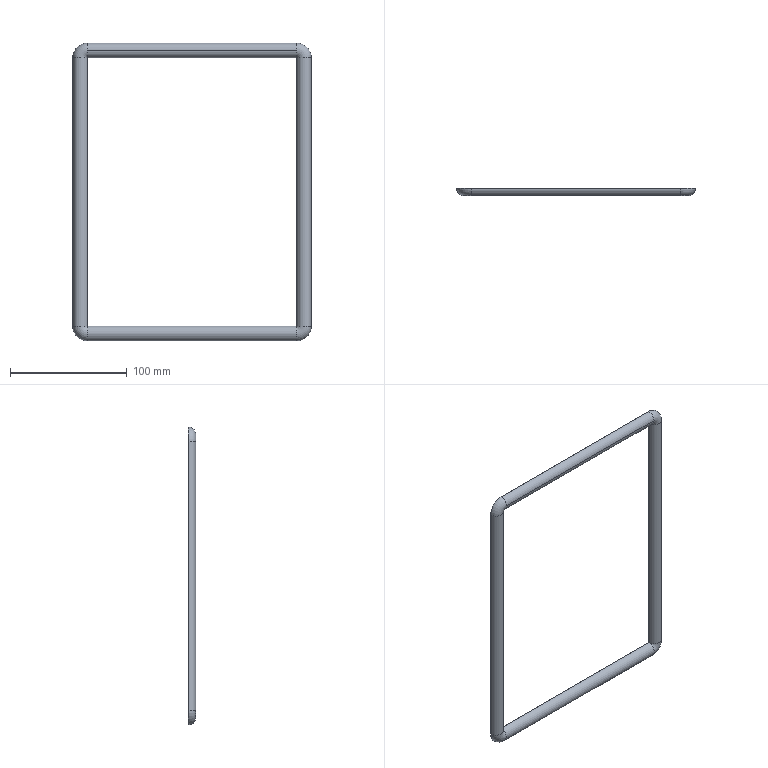Part | SolidWorks | features BaseBody 1 | 1 solid | 43 faces | box 204.775 x 6.35 x 255.575 mm | volume 53856 mm3 | plane 18 | cylinder 13 | cone 8 | torus 4 | commonest cylinder face diameters 12.7 x5 0.051 x4 25.349 x4
STEP:
#1=CARTESIAN_POINT('',(-89.687,-6.35,121.437));
#2=VERTEX_POINT('',#1);
#3=CARTESIAN_POINT('',(-89.687,0.,127.787));
#4=VERTEX_POINT('',#3);
#5=CARTESIAN_POINT('',(-89.687,0.,121.437));
#6=DIRECTION('',(-1.,0.,0.));
#7=DIRECTION('',(0.,0.,-1.));
#8=AXIS2_PLACEMENT_3D('',#5,#6,#7);
#9=CIRCLE('',#8,6.35);
#10=EDGE_CURVE('',#2,#4,#9,.T.);
#11=ORIENTED_EDGE('',*,*,#10,.F.);
#12=CARTESIAN_POINT('',(89.687,-6.35,121.437));
#13=VERTEX_POINT('',#12);
#14=CARTESIAN_POINT('',(-89.687,-6.35,121.437));
#15=DIRECTION('',(1.,0.,0.));
#16=VECTOR('',#15,1000.);
#17=LINE('',#14,#16);
#18=EDGE_CURVE('',#2,#13,#17,.T.);
#19=ORIENTED_EDGE('',*,*,#18,.T.);
#20=CARTESIAN_POINT('',(89.687,0.,127.787));
#21=VERTEX_POINT('',#20);
#22=CARTESIAN_POINT('',(89.687,0.,121.437));
#23=DIRECTION('',(-1.,0.,0.));
#24=DIRECTION('',(0.,0.,-1.));
#25=AXIS2_PLACEMENT_3D('',#22,#23,#24);
#26=CIRCLE('',#25,6.35);
#27=EDGE_CURVE('',#13,#21,#26,.T.);
#28=ORIENTED_EDGE('',*,*,#27,.T.);
#29=CARTESIAN_POINT('',(-89.687,0.,127.787));
#30=DIRECTION('',(1.,0.,0.));
#31=VECTOR('',#30,1000.);
#32=LINE('',#29,#31);
#33=EDGE_CURVE('',#4,#21,#32,.T.);
#34=ORIENTED_EDGE('',*,*,#33,.F.);
#35=EDGE_LOOP('',(#11,#19,#28,#34));
#36=FACE_OUTER_BOUND('',#35,.T.);
#37=CARTESIAN_POINT('',(-89.687,0.,121.437));
#38=DIRECTION('',(1.,0.,0.));
#39=DIRECTION('',(0.,-1.,0.));
#40=AXIS2_PLACEMENT_3D('',#37,#38,#39);
#41=CYLINDRICAL_SURFACE('',#40,6.35);
#42=ADVANCED_FACE('',(#36),#41,.T.);
#43=CARTESIAN_POINT('',(-89.687,0.,-115.087));
#44=VERTEX_POINT('',#43);
#45=CARTESIAN_POINT('',(-89.687,0.,-127.787));
#46=VERTEX_POINT('',#45);
#47=CARTESIAN_POINT('',(-89.687,0.,-121.437));
#48=DIRECTION('',(1.,0.,0.));
#49=DIRECTION('',(0.,0.,1.));
#50=AXIS2_PLACEMENT_3D('',#47,#48,#49);
#51=CIRCLE('',#50,6.35);
#52=EDGE_CURVE('',#44,#46,#51,.T.);
#53=ORIENTED_EDGE('',*,*,#52,.F.);
#54=CARTESIAN_POINT('',(-102.387,0.,-115.087));
#55=VERTEX_POINT('',#54);
#56=CARTESIAN_POINT('',(-96.037,0.,-115.087));
#57=DIRECTION('',(0.,0.,-1.));
#58=DIRECTION('',(1.,0.,0.));
#59=AXIS2_PLACEMENT_3D('',#56,#57,#58);
#60=CIRCLE('',#59,6.35);
#61=EDGE_CURVE('',#44,#55,#60,.T.);
#62=ORIENTED_EDGE('',*,*,#61,.T.);
#63=CARTESIAN_POINT('',(-89.687,0.,-115.087));
#64=DIRECTION('',(0.,1.,0.));
#65=DIRECTION('',(0.,0.,-1.));
#66=AXIS2_PLACEMENT_3D('',#63,#64,#65);
#67=CIRCLE('',#66,12.7);
#68=EDGE_CURVE('',#46,#55,#67,.T.);
#69=ORIENTED_EDGE('',*,*,#68,.F.);
#70=EDGE_LOOP('',(#53,#62,#69));
#71=FACE_OUTER_BOUND('',#70,.T.);
#72=CARTESIAN_POINT('',(-89.687,0.,-115.087));
#73=DIRECTION('',(0.,1.,0.));
#74=DIRECTION('',(1.,0.,0.));
#75=AXIS2_PLACEMENT_3D('',#72,#73,#74);
#76=TOROIDAL_SURFACE('',#75,6.35,6.35);
#77=ADVANCED_FACE('',(#71),#76,.T.);
#78=CARTESIAN_POINT('',(89.687,0.,-115.087));
#79=VERTEX_POINT('',#78);
#80=CARTESIAN_POINT('',(89.687,0.,-115.087));
#81=DIRECTION('',(-1.,0.,0.));
#82=VECTOR('',#81,1000.);
#83=LINE('',#80,#82);
#84=EDGE_CURVE('',#79,#44,#83,.T.);
#85=ORIENTED_EDGE('',*,*,#84,.T.);
#86=ORIENTED_EDGE('',*,*,#52,.T.);
#87=CARTESIAN_POINT('',(89.687,0.,-127.787));
#88=VERTEX_POINT('',#87);
#89=CARTESIAN_POINT('',(89.687,0.,-127.787));
#90=DIRECTION('',(-1.,0.,0.));
#91=VECTOR('',#90,1000.);
#92=LINE('',#89,#91);
#93=EDGE_CURVE('',#88,#46,#92,.T.);
#94=ORIENTED_EDGE('',*,*,#93,.F.);
#95=CARTESIAN_POINT('',(89.687,0.,-121.437));
#96=DIRECTION('',(1.,0.,0.));
#97=DIRECTION('',(0.,0.,1.));
#98=AXIS2_PLACEMENT_3D('',#95,#96,#97);
#99=CIRCLE('',#98,6.35);
#100=EDGE_CURVE('',#79,#88,#99,.T.);
#101=ORIENTED_EDGE('',*,*,#100,.F.);
#102=EDGE_LOOP('',(#85,#86,#94,#101));
#103=FACE_OUTER_BOUND('',#102,.T.);
#104=CARTESIAN_POINT('',(89.687,0.,-121.437));
#105=DIRECTION('',(-1.,0.,0.));
#106=DIRECTION('',(0.,0.,1.));
#107=AXIS2_PLACEMENT_3D('',#104,#105,#106);
#108=CYLINDRICAL_SURFACE('',#107,6.35);
#109=ADVANCED_FACE('',(#103),#108,.T.);
#110=CARTESIAN_POINT('',(102.387,0.,-115.087));
#111=VERTEX_POINT('',#110);
#112=CARTESIAN_POINT('',(96.037,0.,-115.087));
#113=DIRECTION('',(0.,0.,1.));
#114=DIRECTION('',(-1.,0.,0.));
#115=AXIS2_PLACEMENT_3D('',#112,#113,#114);
#116=CIRCLE('',#115,6.35);
#117=EDGE_CURVE('',#79,#111,#116,.T.);
#118=ORIENTED_EDGE('',*,*,#117,.F.);
#119=ORIENTED_EDGE('',*,*,#100,.T.);
#120=CARTESIAN_POINT('',(89.687,0.,-115.087));
#121=DIRECTION('',(0.,1.,0.));
#122=DIRECTION('',(1.,0.,0.));
#123=AXIS2_PLACEMENT_3D('',#120,#121,#122);
#124=CIRCLE('',#123,12.7);
#125=EDGE_CURVE('',#111,#88,#124,.T.);
#126=ORIENTED_EDGE('',*,*,#125,.F.);
#127=EDGE_LOOP('',(#118,#119,#126));
#128=FACE_OUTER_BOUND('',#127,.T.);
#129=CARTESIAN_POINT('',(89.687,0.,-115.087));
#130=DIRECTION('',(0.,1.,0.));
#131=DIRECTION('',(1.,0.,0.));
#132=AXIS2_PLACEMENT_3D('',#129,#130,#131);
#133=TOROIDAL_SURFACE('',#132,6.35,6.35);
#134=ADVANCED_FACE('',(#128),#133,.T.);
#135=CARTESIAN_POINT('',(89.687,0.,115.087));
#136=VERTEX_POINT('',#135);
#137=CARTESIAN_POINT('',(89.687,0.,115.087));
#138=DIRECTION('',(0.,0.,-1.));
#139=VECTOR('',#138,1000.);
#140=LINE('',#137,#139);
#141=EDGE_CURVE('',#136,#79,#140,.T.);
#142=ORIENTED_EDGE('',*,*,#141,.T.);
#143=ORIENTED_EDGE('',*,*,#117,.T.);
#144=CARTESIAN_POINT('',(102.387,0.,115.087));
#145=VERTEX_POINT('',#144);
#146=CARTESIAN_POINT('',(102.387,0.,115.087));
#147=DIRECTION('',(0.,0.,-1.));
#148=VECTOR('',#147,1000.);
#149=LINE('',#146,#148);
#150=EDGE_CURVE('',#145,#111,#149,.T.);
#151=ORIENTED_EDGE('',*,*,#150,.F.);
#152=CARTESIAN_POINT('',(96.037,0.,115.087));
#153=DIRECTION('',(0.,0.,1.));
#154=DIRECTION('',(-1.,0.,0.));
#155=AXIS2_PLACEMENT_3D('',#152,#153,#154);
#156=CIRCLE('',#155,6.35);
#157=EDGE_CURVE('',#136,#145,#156,.T.);
#158=ORIENTED_EDGE('',*,*,#157,.F.);
#159=EDGE_LOOP('',(#142,#143,#151,#158));
#160=FACE_OUTER_BOUND('',#159,.T.);
#161=CARTESIAN_POINT('',(96.037,0.,115.087));
#162=DIRECTION('',(0.,0.,-1.));
#163=DIRECTION('',(-1.,0.,0.));
#164=AXIS2_PLACEMENT_3D('',#161,#162,#163);
#165=CYLINDRICAL_SURFACE('',#164,6.35);
#166=ADVANCED_FACE('',(#160),#165,.T.);
#167=CARTESIAN_POINT('',(89.687,0.,121.437));
#168=DIRECTION('',(-1.,0.,0.));
#169=DIRECTION('',(0.,0.,-1.));
#170=AXIS2_PLACEMENT_3D('',#167,#168,#169);
#171=CIRCLE('',#170,6.35);
#172=EDGE_CURVE('',#136,#13,#171,.T.);
#173=ORIENTED_EDGE('',*,*,#172,.F.);
#174=ORIENTED_EDGE('',*,*,#157,.T.);
#175=CARTESIAN_POINT('',(89.687,0.,115.087));
#176=DIRECTION('',(0.,1.,0.));
#177=DIRECTION('',(0.,0.,1.));
#178=AXIS2_PLACEMENT_3D('',#175,#176,#177);
#179=CIRCLE('',#178,12.7);
#180=EDGE_CURVE('',#21,#145,#179,.T.);
#181=ORIENTED_EDGE('',*,*,#180,.F.);
#182=ORIENTED_EDGE('',*,*,#27,.F.);
#183=EDGE_LOOP('',(#173,#174,#181,#182));
#184=FACE_OUTER_BOUND('',#183,.T.);
#185=CARTESIAN_POINT('',(89.687,0.,115.087));
#186=DIRECTION('',(0.,1.,0.));
#187=DIRECTION('',(1.,0.,0.));
#188=AXIS2_PLACEMENT_3D('',#185,#186,#187);
#189=TOROIDAL_SURFACE('',#188,6.35,6.35);
#190=ADVANCED_FACE('',(#184),#189,.T.);
#191=ORIENTED_EDGE('',*,*,#18,.F.);
#192=CARTESIAN_POINT('',(-89.687,0.,115.087));
#193=VERTEX_POINT('',#192);
#194=CARTESIAN_POINT('',(-89.687,0.,121.437));
#195=DIRECTION('',(-1.,0.,0.));
#196=DIRECTION('',(0.,0.,-1.));
#197=AXIS2_PLACEMENT_3D('',#194,#195,#196);
#198=CIRCLE('',#197,6.35);
#199=EDGE_CURVE('',#193,#2,#198,.T.);
#200=ORIENTED_EDGE('',*,*,#199,.F.);
#201=CARTESIAN_POINT('',(-89.687,0.,115.087));
#202=DIRECTION('',(1.,0.,0.));
#203=VECTOR('',#202,1000.);
#204=LINE('',#201,#203);
#205=EDGE_CURVE('',#193,#136,#204,.T.);
#206=ORIENTED_EDGE('',*,*,#205,.T.);
#207=ORIENTED_EDGE('',*,*,#172,.T.);
#208=EDGE_LOOP('',(#191,#200,#206,#207));
#209=FACE_OUTER_BOUND('',#208,.T.);
#210=CARTESIAN_POINT('',(-89.687,0.,121.437));
#211=DIRECTION('',(1.,0.,0.));
#212=DIRECTION('',(0.,-1.,0.));
#213=AXIS2_PLACEMENT_3D('',#210,#211,#212);
#214=CYLINDRICAL_SURFACE('',#213,6.35);
#215=ADVANCED_FACE('',(#209),#214,.T.);
#216=CARTESIAN_POINT('',(-102.387,0.,115.087));
#217=VERTEX_POINT('',#216);
#218=CARTESIAN_POINT('',(-96.037,0.,115.087));
#219=DIRECTION('',(0.,0.,-1.));
#220=DIRECTION('',(1.,0.,0.));
#221=AXIS2_PLACEMENT_3D('',#218,#219,#220);
#222=CIRCLE('',#221,6.35);
#223=EDGE_CURVE('',#193,#217,#222,.T.);
#224=ORIENTED_EDGE('',*,*,#223,.F.);
#225=ORIENTED_EDGE('',*,*,#199,.T.);
#226=ORIENTED_EDGE('',*,*,#10,.T.);
#227=CARTESIAN_POINT('',(-89.687,0.,115.087));
#228=DIRECTION('',(0.,1.,0.));
#229=DIRECTION('',(-1.,0.,0.));
#230=AXIS2_PLACEMENT_3D('',#227,#228,#229);
#231=CIRCLE('',#230,12.7);
#232=EDGE_CURVE('',#217,#4,#231,.T.);
#233=ORIENTED_EDGE('',*,*,#232,.F.);
#234=EDGE_LOOP('',(#224,#225,#226,#233));
#235=FACE_OUTER_BOUND('',#234,.T.);
#236=CARTESIAN_POINT('',(-89.687,0.,115.087));
#237=DIRECTION('',(0.,1.,0.));
#238=DIRECTION('',(1.,0.,0.));
#239=AXIS2_PLACEMENT_3D('',#236,#237,#238);
#240=TOROIDAL_SURFACE('',#239,6.35,6.35);
#241=ADVANCED_FACE('',(#235),#240,.T.);
#242=CARTESIAN_POINT('',(-102.387,0.,-115.087));
#243=DIRECTION('',(0.,0.,1.));
#244=VECTOR('',#243,1000.);
#245=LINE('',#242,#244);
#246=EDGE_CURVE('',#55,#217,#245,.T.);
#247=ORIENTED_EDGE('',*,*,#246,.T.);
#248=ORIENTED_EDGE('',*,*,#232,.T.);
#249=ORIENTED_EDGE('',*,*,#33,.T.);
#250=ORIENTED_EDGE('',*,*,#180,.T.);
#251=ORIENTED_EDGE('',*,*,#150,.T.);
#252=ORIENTED_EDGE('',*,*,#125,.T.);
#253=ORIENTED_EDGE('',*,*,#93,.T.);
#254=ORIENTED_EDGE('',*,*,#68,.T.);
#255=EDGE_LOOP('',(#247,#248,#249,#250,#251,#252,#253,#254));
#256=FACE_OUTER_BOUND('',#255,.T.);
#257=ORIENTED_EDGE('',*,*,#205,.F.);
#258=CARTESIAN_POINT('',(-89.687,0.,-115.087));
#259=DIRECTION('',(0.,0.,1.));
#260=VECTOR('',#259,1000.);
#261=LINE('',#258,#260);
#262=EDGE_CURVE('',#44,#193,#261,.T.);
#263=ORIENTED_EDGE('',*,*,#262,.F.);
#264=ORIENTED_EDGE('',*,*,#84,.F.);
#265=ORIENTED_EDGE('',*,*,#141,.F.);
#266=EDGE_LOOP('',(#257,#263,#264,#265));
#267=FACE_BOUND('',#266,.T.);
#268=CARTESIAN_POINT('',(-102.387,0.,-115.087));
#269=DIRECTION('',(0.,1.,0.));
#270=DIRECTION('',(1.,0.,0.));
#271=AXIS2_PLACEMENT_3D('',#268,#269,#270);
#272=PLANE('',#271);
#273=ADVANCED_FACE('',(#256,#267),#272,.T.);
#274=ORIENTED_EDGE('',*,*,#262,.T.);
#275=ORIENTED_EDGE('',*,*,#223,.T.);
#276=ORIENTED_EDGE('',*,*,#246,.F.);
#277=ORIENTED_EDGE('',*,*,#61,.F.);
#278=EDGE_LOOP('',(#274,#275,#276,#277));
#279=FACE_OUTER_BOUND('',#278,.T.);
#280=CARTESIAN_POINT('',(-96.037,0.,-115.087));
#281=DIRECTION('',(0.,0.,1.));
#282=DIRECTION('',(1.,0.,0.));
#283=AXIS2_PLACEMENT_3D('',#280,#281,#282);
#284=CYLINDRICAL_SURFACE('',#283,6.35);
#285=ADVANCED_FACE('',(#279),#284,.T.);
#286=CLOSED_SHELL('',(#42,#77,#109,#134,#166,#190,#215,#241,#273,#285));
#287=CARTESIAN_POINT('',(102.362,-0.0508,115.087));
#288=VERTEX_POINT('',#287);
#289=CARTESIAN_POINT('',(96.037,-0.1016,115.087));
#290=VERTEX_POINT('',#289);
#291=CARTESIAN_POINT('',(102.362,-0.0508,115.087));
#292=DIRECTION('',(-1.,-0.008032,0.));
#293=VECTOR('',#292,1000.);
#294=LINE('',#291,#293);
#295=EDGE_CURVE('',#288,#290,#294,.T.);
#296=ORIENTED_EDGE('',*,*,#295,.F.);
#297=CARTESIAN_POINT('',(102.362,-0.0508,-115.087));
#298=VERTEX_POINT('',#297);
#299=CARTESIAN_POINT('',(102.362,-0.0508,115.087));
#300=DIRECTION('',(0.,0.,-1.));
#301=VECTOR('',#300,1000.);
#302=LINE('',#299,#301);
#303=EDGE_CURVE('',#288,#298,#302,.T.);
#304=ORIENTED_EDGE('',*,*,#303,.T.);
#305=CARTESIAN_POINT('',(96.037,-0.1016,-115.087));
#306=VERTEX_POINT('',#305);
#307=CARTESIAN_POINT('',(102.362,-0.0508,-115.087));
#308=DIRECTION('',(-1.,-0.008032,0.));
#309=VECTOR('',#308,1000.);
#310=LINE('',#307,#309);
#311=EDGE_CURVE('',#298,#306,#310,.T.);
#312=ORIENTED_EDGE('',*,*,#311,.T.);
#313=CARTESIAN_POINT('',(96.037,-0.1016,115.087));
#314=DIRECTION('',(0.,0.,-1.));
#315=VECTOR('',#314,1000.);
#316=LINE('',#313,#315);
#317=EDGE_CURVE('',#290,#306,#316,.T.);
#318=ORIENTED_EDGE('',*,*,#317,.F.);
#319=EDGE_LOOP('',(#296,#304,#312,#318));
#320=FACE_OUTER_BOUND('',#319,.T.);
#321=CARTESIAN_POINT('',(102.362,-0.0508,115.087));
#322=DIRECTION('',(-0.008032,1.,0.));
#323=DIRECTION('',(0.,0.,1.));
#324=AXIS2_PLACEMENT_3D('',#321,#322,#323);
#325=PLANE('',#324);
#326=ADVANCED_FACE('',(#320),#325,.T.);
#327=CARTESIAN_POINT('',(89.713,-0.0508,115.087));
#328=VERTEX_POINT('',#327);
#329=CARTESIAN_POINT('',(96.037,-0.1016,115.087));
#330=DIRECTION('',(-1.,0.008032,0.));
#331=VECTOR('',#330,1000.);
#332=LINE('',#329,#331);
#333=EDGE_CURVE('',#290,#328,#332,.T.);
#334=ORIENTED_EDGE('',*,*,#333,.F.);
#335=ORIENTED_EDGE('',*,*,#317,.T.);
#336=CARTESIAN_POINT('',(89.713,-0.0508,-115.087));
#337=VERTEX_POINT('',#336);
#338=CARTESIAN_POINT('',(96.037,-0.1016,-115.087));
#339=DIRECTION('',(-1.,0.008032,0.));
#340=VECTOR('',#339,1000.);
#341=LINE('',#338,#340);
#342=EDGE_CURVE('',#306,#337,#341,.T.);
#343=ORIENTED_EDGE('',*,*,#342,.T.);
#344=CARTESIAN_POINT('',(89.713,-0.0508,115.087));
#345=DIRECTION('',(0.,0.,-1.));
#346=VECTOR('',#345,1000.);
#347=LINE('',#344,#346);
#348=EDGE_CURVE('',#328,#337,#347,.T.);
#349=ORIENTED_EDGE('',*,*,#348,.F.);
#350=EDGE_LOOP('',(#334,#335,#343,#349));
#351=FACE_OUTER_BOUND('',#350,.T.);
#352=CARTESIAN_POINT('',(96.037,-0.1016,115.087));
#353=DIRECTION('',(0.008032,1.,0.));
#354=DIRECTION('',(0.,0.,-1.));
#355=AXIS2_PLACEMENT_3D('',#352,#353,#354);
#356=PLANE('',#355);
#357=ADVANCED_FACE('',(#351),#356,.T.);
#358=CARTESIAN_POINT('',(89.713,-0.0254,115.087));
#359=VERTEX_POINT('',#358);
#360=CARTESIAN_POINT('',(89.713,-0.0508,115.087));
#361=DIRECTION('',(0.,1.,0.));
#362=VECTOR('',#361,1000.);
#363=LINE('',#360,#362);
#364=EDGE_CURVE('',#328,#359,#363,.T.);
#365=ORIENTED_EDGE('',*,*,#364,.F.);
#366=ORIENTED_EDGE('',*,*,#348,.T.);
#367=CARTESIAN_POINT('',(89.713,-0.0254,-115.087));
#368=VERTEX_POINT('',#367);
#369=CARTESIAN_POINT('',(89.713,-0.0508,-115.087));
#370=DIRECTION('',(0.,1.,0.));
#371=VECTOR('',#370,1000.);
#372=LINE('',#369,#371);
#373=EDGE_CURVE('',#337,#368,#372,.T.);
#374=ORIENTED_EDGE('',*,*,#373,.T.);
#375=CARTESIAN_POINT('',(89.713,-0.0254,115.087));
#376=DIRECTION('',(0.,0.,-1.));
#377=VECTOR('',#376,1000.);
#378=LINE('',#375,#377);
#379=EDGE_CURVE('',#359,#368,#378,.T.);
#380=ORIENTED_EDGE('',*,*,#379,.F.);
#381=EDGE_LOOP('',(#365,#366,#374,#380));
#382=FACE_OUTER_BOUND('',#381,.T.);
#383=CARTESIAN_POINT('',(89.713,-0.0508,115.087));
#384=DIRECTION('',(1.,0.,0.));
#385=DIRECTION('',(0.,0.,1.));
#386=AXIS2_PLACEMENT_3D('',#383,#384,#385);
#387=PLANE('',#386);
#388=ADVANCED_FACE('',(#382),#387,.T.);
#389=CARTESIAN_POINT('',(89.687,-0.0254,127.762));
#390=VERTEX_POINT('',#389);
#391=CARTESIAN_POINT('',(89.687,-0.0508,127.762));
#392=VERTEX_POINT('',#391);
#393=CARTESIAN_POINT('',(89.687,-0.0254,127.762));
#394=DIRECTION('',(0.,-1.,0.));
#395=VECTOR('',#394,1000.);
#396=LINE('',#393,#395);
#397=EDGE_CURVE('',#390,#392,#396,.T.);
#398=ORIENTED_EDGE('',*,*,#397,.F.);
#399=CARTESIAN_POINT('',(102.362,-0.0254,115.087));
#400=VERTEX_POINT('',#399);
#401=CARTESIAN_POINT('',(89.687,-0.0254,115.087));
#402=DIRECTION('',(0.,1.,0.));
#403=DIRECTION('',(0.,0.,1.));
#404=AXIS2_PLACEMENT_3D('',#401,#402,#403);
#405=CIRCLE('',#404,12.675);
#406=EDGE_CURVE('',#390,#400,#405,.T.);
#407=ORIENTED_EDGE('',*,*,#406,.T.);
#408=CARTESIAN_POINT('',(102.362,-0.0254,115.087));
#409=DIRECTION('',(0.,-1.,0.));
#410=VECTOR('',#409,1000.);
#411=LINE('',#408,#410);
#412=EDGE_CURVE('',#400,#288,#411,.T.);
#413=ORIENTED_EDGE('',*,*,#412,.T.);
#414=CARTESIAN_POINT('',(89.687,-0.0508,115.087));
#415=DIRECTION('',(0.,1.,0.));
#416=DIRECTION('',(0.,0.,1.));
#417=AXIS2_PLACEMENT_3D('',#414,#415,#416);
#418=CIRCLE('',#417,12.675);
#419=EDGE_CURVE('',#392,#288,#418,.T.);
#420=ORIENTED_EDGE('',*,*,#419,.F.);
#421=EDGE_LOOP('',(#398,#407,#413,#420));
#422=FACE_OUTER_BOUND('',#421,.T.);
#423=CARTESIAN_POINT('',(89.687,0.,115.087));
#424=DIRECTION('',(0.,1.,0.));
#425=DIRECTION('',(1.,0.,0.));
#426=AXIS2_PLACEMENT_3D('',#423,#424,#425);
#427=CYLINDRICAL_SURFACE('',#426,12.675);
#428=ADVANCED_FACE('',(#422),#427,.F.);
#429=CARTESIAN_POINT('',(89.687,-0.1016,121.437));
#430=VERTEX_POINT('',#429);
#431=CARTESIAN_POINT('',(89.687,-0.0508,127.762));
#432=DIRECTION('',(0.,-0.008032,-1.));
#433=VECTOR('',#432,1000.);
#434=LINE('',#431,#433);
#435=EDGE_CURVE('',#392,#430,#434,.T.);
#436=ORIENTED_EDGE('',*,*,#435,.F.);
#437=ORIENTED_EDGE('',*,*,#419,.T.);
#438=ORIENTED_EDGE('',*,*,#295,.T.);
#439=CARTESIAN_POINT('',(89.687,-0.1016,115.087));
#440=DIRECTION('',(0.,1.,0.));
#441=DIRECTION('',(0.,0.,1.));
#442=AXIS2_PLACEMENT_3D('',#439,#440,#441);
#443=CIRCLE('',#442,6.35);
#444=EDGE_CURVE('',#430,#290,#443,.T.);
#445=ORIENTED_EDGE('',*,*,#444,.F.);
#446=EDGE_LOOP('',(#436,#437,#438,#445));
#447=FACE_OUTER_BOUND('',#446,.T.);
#448=CARTESIAN_POINT('',(89.687,-0.1016,115.087));
#449=DIRECTION('',(0.,1.,0.));
#450=DIRECTION('',(1.,0.,0.));
#451=AXIS2_PLACEMENT_3D('',#448,#449,#450);
#452=CONICAL_SURFACE('',#451,6.35,1.563);
#453=ADVANCED_FACE('',(#447),#452,.F.);
#454=CARTESIAN_POINT('',(89.687,-0.0508,115.113));
#455=VERTEX_POINT('',#454);
#456=CARTESIAN_POINT('',(89.687,-0.1016,121.437));
#457=DIRECTION('',(0.,0.008032,-1.));
#458=VECTOR('',#457,1000.);
#459=LINE('',#456,#458);
#460=EDGE_CURVE('',#430,#455,#459,.T.);
#461=ORIENTED_EDGE('',*,*,#460,.F.);
#462=ORIENTED_EDGE('',*,*,#444,.T.);
#463=ORIENTED_EDGE('',*,*,#333,.T.);
#464=CARTESIAN_POINT('',(89.687,-0.0508,115.087));
#465=DIRECTION('',(0.,1.,0.));
#466=DIRECTION('',(0.,0.,1.));
#467=AXIS2_PLACEMENT_3D('',#464,#465,#466);
#468=CIRCLE('',#467,0.0254);
#469=EDGE_CURVE('',#455,#328,#468,.T.);
#470=ORIENTED_EDGE('',*,*,#469,.F.);
#471=EDGE_LOOP('',(#461,#462,#463,#470));
#472=FACE_OUTER_BOUND('',#471,.T.);
#473=CARTESIAN_POINT('',(89.687,-0.0508,115.087));
#474=DIRECTION('',(0.,-1.,0.));
#475=DIRECTION('',(-1.,0.,0.));
#476=AXIS2_PLACEMENT_3D('',#473,#474,#475);
#477=CONICAL_SURFACE('',#476,0.0254,1.563);
#478=ADVANCED_FACE('',(#472),#477,.T.);
#479=CARTESIAN_POINT('',(89.687,-0.0254,115.113));
#480=VERTEX_POINT('',#479);
#481=CARTESIAN_POINT('',(89.687,-0.0508,115.113));
#482=DIRECTION('',(0.,1.,0.));
#483=VECTOR('',#482,1000.);
#484=LINE('',#481,#483);
#485=EDGE_CURVE('',#455,#480,#484,.T.);
#486=ORIENTED_EDGE('',*,*,#485,.F.);
#487=ORIENTED_EDGE('',*,*,#469,.T.);
#488=ORIENTED_EDGE('',*,*,#364,.T.);
#489=CARTESIAN_POINT('',(89.687,-0.0254,115.087));
#490=DIRECTION('',(0.,1.,0.));
#491=DIRECTION('',(0.,0.,1.));
#492=AXIS2_PLACEMENT_3D('',#489,#490,#491);
#493=CIRCLE('',#492,0.0254);
#494=EDGE_CURVE('',#480,#359,#493,.T.);
#495=ORIENTED_EDGE('',*,*,#494,.F.);
#496=EDGE_LOOP('',(#486,#487,#488,#495));
#497=FACE_OUTER_BOUND('',#496,.T.);
#498=CARTESIAN_POINT('',(89.687,0.,115.087));
#499=DIRECTION('',(0.,1.,0.));
#500=DIRECTION('',(1.,0.,0.));
#501=AXIS2_PLACEMENT_3D('',#498,#499,#500);
#502=CYLINDRICAL_SURFACE('',#501,0.0254);
#503=ADVANCED_FACE('',(#497),#502,.T.);
#504=CARTESIAN_POINT('',(-89.687,-0.0254,127.762));
#505=VERTEX_POINT('',#504);
#506=CARTESIAN_POINT('',(-89.687,-0.0508,127.762));
#507=VERTEX_POINT('',#506);
#508=CARTESIAN_POINT('',(-89.687,-0.0254,127.762));
#509=DIRECTION('',(0.,-1.,0.));
#510=VECTOR('',#509,1000.);
#511=LINE('',#508,#510);
#512=EDGE_CURVE('',#505,#507,#511,.T.);
#513=ORIENTED_EDGE('',*,*,#512,.F.);
#514=CARTESIAN_POINT('',(-89.687,-0.0254,127.762));
#515=DIRECTION('',(1.,0.,0.));
#516=VECTOR('',#515,1000.);
#517=LINE('',#514,#516);
#518=EDGE_CURVE('',#505,#390,#517,.T.);
#519=ORIENTED_EDGE('',*,*,#518,.T.);
#520=ORIENTED_EDGE('',*,*,#397,.T.);
#521=CARTESIAN_POINT('',(-89.687,-0.0508,127.762));
#522=DIRECTION('',(1.,0.,0.));
#523=VECTOR('',#522,1000.);
#524=LINE('',#521,#523);
#525=EDGE_CURVE('',#507,#392,#524,.T.);
#526=ORIENTED_EDGE('',*,*,#525,.F.);
#527=EDGE_LOOP('',(#513,#519,#520,#526));
#528=FACE_OUTER_BOUND('',#527,.T.);
#529=CARTESIAN_POINT('',(-89.687,-0.0254,127.762));
#530=DIRECTION('',(0.,0.,-1.));
#531=DIRECTION('',(0.,-1.,0.));
#532=AXIS2_PLACEMENT_3D('',#529,#530,#531);
#533=PLANE('',#532);
#534=ADVANCED_FACE('',(#528),#533,.T.);
#535=CARTESIAN_POINT('',(-89.687,-0.1016,121.437));
#536=VERTEX_POINT('',#535);
#537=CARTESIAN_POINT('',(-89.687,-0.0508,127.762));
#538=DIRECTION('',(0.,-0.008032,-1.));
#539=VECTOR('',#538,1000.);
#540=LINE('',#537,#539);
#541=EDGE_CURVE('',#507,#536,#540,.T.);
#542=ORIENTED_EDGE('',*,*,#541,.F.);
#543=ORIENTED_EDGE('',*,*,#525,.T.);
#544=ORIENTED_EDGE('',*,*,#435,.T.);
#545=CARTESIAN_POINT('',(-89.687,-0.1016,121.437));
#546=DIRECTION('',(1.,0.,0.));
#547=VECTOR('',#546,1000.);
#548=LINE('',#545,#547);
#549=EDGE_CURVE('',#536,#430,#548,.T.);
#550=ORIENTED_EDGE('',*,*,#549,.F.);
#551=EDGE_LOOP('',(#542,#543,#544,#550));
#552=FACE_OUTER_BOUND('',#551,.T.);
#553=CARTESIAN_POINT('',(-89.687,-0.0508,127.762));
#554=DIRECTION('',(0.,1.,-0.008032));
#555=DIRECTION('',(-1.,0.,0.));
#556=AXIS2_PLACEMENT_3D('',#553,#554,#555);
#557=PLANE('',#556);
#558=ADVANCED_FACE('',(#552),#557,.T.);
#559=CARTESIAN_POINT('',(-89.687,-0.0508,115.113));
#560=VERTEX_POINT('',#559);
#561=CARTESIAN_POINT('',(-89.687,-0.1016,121.437));
#562=DIRECTION('',(0.,0.008032,-1.));
#563=VECTOR('',#562,1000.);
#564=LINE('',#561,#563);
#565=EDGE_CURVE('',#536,#560,#564,.T.);
#566=ORIENTED_EDGE('',*,*,#565,.F.);
#567=ORIENTED_EDGE('',*,*,#549,.T.);
#568=ORIENTED_EDGE('',*,*,#460,.T.);
#569=CARTESIAN_POINT('',(-89.687,-0.0508,115.113));
#570=DIRECTION('',(1.,0.,0.));
#571=VECTOR('',#570,1000.);
#572=LINE('',#569,#571);
#573=EDGE_CURVE('',#560,#455,#572,.T.);
#574=ORIENTED_EDGE('',*,*,#573,.F.);
#575=EDGE_LOOP('',(#566,#567,#568,#574));
#576=FACE_OUTER_BOUND('',#575,.T.);
#577=CARTESIAN_POINT('',(-89.687,-0.1016,121.437));
#578=DIRECTION('',(0.,1.,0.008032));
#579=DIRECTION('',(1.,0.,0.));
#580=AXIS2_PLACEMENT_3D('',#577,#578,#579);
#581=PLANE('',#580);
#582=ADVANCED_FACE('',(#576),#581,.T.);
#583=CARTESIAN_POINT('',(-89.687,-0.0254,115.113));
#584=VERTEX_POINT('',#583);
#585=CARTESIAN_POINT('',(-89.687,-0.0508,115.113));
#586=DIRECTION('',(0.,1.,0.));
#587=VECTOR('',#586,1000.);
#588=LINE('',#585,#587);
#589=EDGE_CURVE('',#560,#584,#588,.T.);
#590=ORIENTED_EDGE('',*,*,#589,.F.);
#591=ORIENTED_EDGE('',*,*,#573,.T.);
#592=ORIENTED_EDGE('',*,*,#485,.T.);
#593=CARTESIAN_POINT('',(-89.687,-0.0254,115.113));
#594=DIRECTION('',(1.,0.,0.));
#595=VECTOR('',#594,1000.);
#596=LINE('',#593,#595);
#597=EDGE_CURVE('',#584,#480,#596,.T.);
#598=ORIENTED_EDGE('',*,*,#597,.F.);
#599=EDGE_LOOP('',(#590,#591,#592,#598));
#600=FACE_OUTER_BOUND('',#599,.T.);
#601=CARTESIAN_POINT('',(-89.687,-0.0508,115.113));
#602=DIRECTION('',(0.,0.,1.));
#603=DIRECTION('',(1.,0.,0.));
#604=AXIS2_PLACEMENT_3D('',#601,#602,#603);
#605=PLANE('',#604);
#606=ADVANCED_FACE('',(#600),#605,.T.);
#607=CARTESIAN_POINT('',(-102.362,-0.0254,115.087));
#608=VERTEX_POINT('',#607);
#609=CARTESIAN_POINT('',(-102.362,-0.0508,115.087));
#610=VERTEX_POINT('',#609);
#611=CARTESIAN_POINT('',(-102.362,-0.0254,115.087));
#612=DIRECTION('',(0.,-1.,0.));
#613=VECTOR('',#612,1000.);
#614=LINE('',#611,#613);
#615=EDGE_CURVE('',#608,#610,#614,.T.);
#616=ORIENTED_EDGE('',*,*,#615,.F.);
#617=CARTESIAN_POINT('',(-89.687,-0.0254,115.087));
#618=DIRECTION('',(0.,1.,0.));
#619=DIRECTION('',(-1.,0.,0.));
#620=AXIS2_PLACEMENT_3D('',#617,#618,#619);
#621=CIRCLE('',#620,12.675);
#622=EDGE_CURVE('',#608,#505,#621,.T.);
#623=ORIENTED_EDGE('',*,*,#622,.T.);
#624=ORIENTED_EDGE('',*,*,#512,.T.);
#625=CARTESIAN_POINT('',(-89.687,-0.0508,115.087));
#626=DIRECTION('',(0.,1.,0.));
#627=DIRECTION('',(-1.,0.,0.));
#628=AXIS2_PLACEMENT_3D('',#625,#626,#627);
#629=CIRCLE('',#628,12.675);
#630=EDGE_CURVE('',#610,#507,#629,.T.);
#631=ORIENTED_EDGE('',*,*,#630,.F.);
#632=EDGE_LOOP('',(#616,#623,#624,#631));
#633=FACE_OUTER_BOUND('',#632,.T.);
#634=CARTESIAN_POINT('',(-89.687,0.,115.087));
#635=DIRECTION('',(0.,1.,0.));
#636=DIRECTION('',(1.,0.,0.));
#637=AXIS2_PLACEMENT_3D('',#634,#635,#636);
#638=CYLINDRICAL_SURFACE('',#637,12.675);
#639=ADVANCED_FACE('',(#633),#638,.F.);
#640=CARTESIAN_POINT('',(-96.037,-0.1016,115.087));
#641=VERTEX_POINT('',#640);
#642=CARTESIAN_POINT('',(-102.362,-0.0508,115.087));
#643=DIRECTION('',(1.,-0.008032,0.));
#644=VECTOR('',#643,1000.);
#645=LINE('',#642,#644);
#646=EDGE_CURVE('',#610,#641,#645,.T.);
#647=ORIENTED_EDGE('',*,*,#646,.F.);
#648=ORIENTED_EDGE('',*,*,#630,.T.);
#649=ORIENTED_EDGE('',*,*,#541,.T.);
#650=CARTESIAN_POINT('',(-89.687,-0.1016,115.087));
#651=DIRECTION('',(0.,1.,0.));
#652=DIRECTION('',(-1.,0.,0.));
#653=AXIS2_PLACEMENT_3D('',#650,#651,#652);
#654=CIRCLE('',#653,6.35);
#655=EDGE_CURVE('',#641,#536,#654,.T.);
#656=ORIENTED_EDGE('',*,*,#655,.F.);
#657=EDGE_LOOP('',(#647,#648,#649,#656));
#658=FACE_OUTER_BOUND('',#657,.T.);
#659=CARTESIAN_POINT('',(-89.687,-0.1016,115.087));
#660=DIRECTION('',(0.,1.,0.));
#661=DIRECTION('',(1.,0.,0.));
#662=AXIS2_PLACEMENT_3D('',#659,#660,#661);
#663=CONICAL_SURFACE('',#662,6.35,1.563);
#664=ADVANCED_FACE('',(#658),#663,.F.);
#665=CARTESIAN_POINT('',(-89.713,-0.0508,115.087));
#666=VERTEX_POINT('',#665);
#667=CARTESIAN_POINT('',(-96.037,-0.1016,115.087));
#668=DIRECTION('',(1.,0.008032,0.));
#669=VECTOR('',#668,1000.);
#670=LINE('',#667,#669);
#671=EDGE_CURVE('',#641,#666,#670,.T.);
#672=ORIENTED_EDGE('',*,*,#671,.F.);
#673=ORIENTED_EDGE('',*,*,#655,.T.);
#674=ORIENTED_EDGE('',*,*,#565,.T.);
#675=CARTESIAN_POINT('',(-89.687,-0.0508,115.087));
#676=DIRECTION('',(0.,1.,0.));
#677=DIRECTION('',(-1.,0.,0.));
#678=AXIS2_PLACEMENT_3D('',#675,#676,#677);
#679=CIRCLE('',#678,0.0254);
#680=EDGE_CURVE('',#666,#560,#679,.T.);
#681=ORIENTED_EDGE('',*,*,#680,.F.);
#682=EDGE_LOOP('',(#672,#673,#674,#681));
#683=FACE_OUTER_BOUND('',#682,.T.);
#684=CARTESIAN_POINT('',(-89.687,-0.0508,115.087));
#685=DIRECTION('',(0.,-1.,0.));
#686=DIRECTION('',(-1.,0.,0.));
#687=AXIS2_PLACEMENT_3D('',#684,#685,#686);
#688=CONICAL_SURFACE('',#687,0.0254,1.563);
#689=ADVANCED_FACE('',(#683),#688,.T.);
#690=CARTESIAN_POINT('',(-89.713,-0.0254,115.087));
#691=VERTEX_POINT('',#690);
#692=CARTESIAN_POINT('',(-89.713,-0.0508,115.087));
#693=DIRECTION('',(0.,1.,0.));
#694=VECTOR('',#693,1000.);
#695=LINE('',#692,#694);
#696=EDGE_CURVE('',#666,#691,#695,.T.);
#697=ORIENTED_EDGE('',*,*,#696,.F.);
#698=ORIENTED_EDGE('',*,*,#680,.T.);
#699=ORIENTED_EDGE('',*,*,#589,.T.);
#700=CARTESIAN_POINT('',(-89.687,-0.0254,115.087));
#701=DIRECTION('',(0.,1.,0.));
#702=DIRECTION('',(-1.,0.,0.));
#703=AXIS2_PLACEMENT_3D('',#700,#701,#702);
#704=CIRCLE('',#703,0.0254);
#705=EDGE_CURVE('',#691,#584,#704,.T.);
#706=ORIENTED_EDGE('',*,*,#705,.F.);
#707=EDGE_LOOP('',(#697,#698,#699,#706));
#708=FACE_OUTER_BOUND('',#707,.T.);
#709=CARTESIAN_POINT('',(-89.687,0.,115.087));
#710=DIRECTION('',(0.,1.,0.));
#711=DIRECTION('',(1.,0.,0.));
#712=AXIS2_PLACEMENT_3D('',#709,#710,#711);
#713=CYLINDRICAL_SURFACE('',#712,0.0254);
#714=ADVANCED_FACE('',(#708),#713,.T.);
#715=CARTESIAN_POINT('',(-89.713,-0.0254,-115.087));
#716=VERTEX_POINT('',#715);
#717=CARTESIAN_POINT('',(-89.713,-0.0254,-115.087));
#718=DIRECTION('',(0.,0.,1.));
#719=VECTOR('',#718,1000.);
#720=LINE('',#717,#719);
#721=EDGE_CURVE('',#716,#691,#720,.T.);
#722=ORIENTED_EDGE('',*,*,#721,.T.);
#723=ORIENTED_EDGE('',*,*,#705,.T.);
#724=ORIENTED_EDGE('',*,*,#597,.T.);
#725=ORIENTED_EDGE('',*,*,#494,.T.);
#726=ORIENTED_EDGE('',*,*,#379,.T.);
#727=CARTESIAN_POINT('',(89.687,-0.0254,-115.113));
#728=VERTEX_POINT('',#727);
#729=CARTESIAN_POINT('',(89.687,-0.0254,-115.087));
#730=DIRECTION('',(0.,1.,0.));
#731=DIRECTION('',(1.,0.,0.));
#732=AXIS2_PLACEMENT_3D('',#729,#730,#731);
#733=CIRCLE('',#732,0.0254);
#734=EDGE_CURVE('',#368,#728,#733,.T.);
#735=ORIENTED_EDGE('',*,*,#734,.T.);
#736=CARTESIAN_POINT('',(-89.687,-0.0254,-115.113));
#737=VERTEX_POINT('',#736);
#738=CARTESIAN_POINT('',(89.687,-0.0254,-115.113));
#739=DIRECTION('',(-1.,0.,0.));
#740=VECTOR('',#739,1000.);
#741=LINE('',#738,#740);
#742=EDGE_CURVE('',#728,#737,#741,.T.);
#743=ORIENTED_EDGE('',*,*,#742,.T.);
#744=CARTESIAN_POINT('',(-89.687,-0.0254,-115.087));
#745=DIRECTION('',(0.,1.,0.));
#746=DIRECTION('',(0.,0.,-1.));
#747=AXIS2_PLACEMENT_3D('',#744,#745,#746);
#748=CIRCLE('',#747,0.0254);
#749=EDGE_CURVE('',#737,#716,#748,.T.);
#750=ORIENTED_EDGE('',*,*,#749,.T.);
#751=EDGE_LOOP('',(#722,#723,#724,#725,#726,#735,#743,#750));
#752=FACE_BOUND('',#751,.T.);
#753=ORIENTED_EDGE('',*,*,#622,.F.);
#754=CARTESIAN_POINT('',(-102.362,-0.0254,-115.087));
#755=VERTEX_POINT('',#754);
#756=CARTESIAN_POINT('',(-102.362,-0.0254,-115.087));
#757=DIRECTION('',(0.,0.,1.));
#758=VECTOR('',#757,1000.);
#759=LINE('',#756,#758);
#760=EDGE_CURVE('',#755,#608,#759,.T.);
#761=ORIENTED_EDGE('',*,*,#760,.F.);
#762=CARTESIAN_POINT('',(-89.687,-0.0254,-127.762));
#763=VERTEX_POINT('',#762);
#764=CARTESIAN_POINT('',(-89.687,-0.0254,-115.087));
#765=DIRECTION('',(0.,1.,0.));
#766=DIRECTION('',(0.,0.,-1.));
#767=AXIS2_PLACEMENT_3D('',#764,#765,#766);
#768=CIRCLE('',#767,12.675);
#769=EDGE_CURVE('',#763,#755,#768,.T.);
#770=ORIENTED_EDGE('',*,*,#769,.F.);
#771=CARTESIAN_POINT('',(89.687,-0.0254,-127.762));
#772=VERTEX_POINT('',#771);
#773=CARTESIAN_POINT('',(89.687,-0.0254,-127.762));
#774=DIRECTION('',(-1.,0.,0.));
#775=VECTOR('',#774,1000.);
#776=LINE('',#773,#775);
#777=EDGE_CURVE('',#772,#763,#776,.T.);
#778=ORIENTED_EDGE('',*,*,#777,.F.);
#779=CARTESIAN_POINT('',(102.362,-0.0254,-115.087));
#780=VERTEX_POINT('',#779);
#781=CARTESIAN_POINT('',(89.687,-0.0254,-115.087));
#782=DIRECTION('',(0.,1.,0.));
#783=DIRECTION('',(1.,0.,0.));
#784=AXIS2_PLACEMENT_3D('',#781,#782,#783);
#785=CIRCLE('',#784,12.675);
#786=EDGE_CURVE('',#780,#772,#785,.T.);
#787=ORIENTED_EDGE('',*,*,#786,.F.);
#788=CARTESIAN_POINT('',(102.362,-0.0254,115.087));
#789=DIRECTION('',(0.,0.,-1.));
#790=VECTOR('',#789,1000.);
#791=LINE('',#788,#790);
#792=EDGE_CURVE('',#400,#780,#791,.T.);
#793=ORIENTED_EDGE('',*,*,#792,.F.);
#794=ORIENTED_EDGE('',*,*,#406,.F.);
#795=ORIENTED_EDGE('',*,*,#518,.F.);
#796=EDGE_LOOP('',(#753,#761,#770,#778,#787,#793,#794,#795));
#797=FACE_OUTER_BOUND('',#796,.T.);
#798=CARTESIAN_POINT('',(-89.713,-0.0254,-115.087));
#799=DIRECTION('',(0.,-1.,0.));
#800=DIRECTION('',(0.,0.,-1.));
#801=AXIS2_PLACEMENT_3D('',#798,#799,#800);
#802=PLANE('',#801);
#803=ADVANCED_FACE('',(#752,#797),#802,.T.);
#804=CARTESIAN_POINT('',(-102.362,-0.0508,-115.087));
#805=VERTEX_POINT('',#804);
#806=CARTESIAN_POINT('',(-102.362,-0.0254,-115.087));
#807=DIRECTION('',(0.,-1.,0.));
#808=VECTOR('',#807,1000.);
#809=LINE('',#806,#808);
#810=EDGE_CURVE('',#755,#805,#809,.T.);
#811=ORIENTED_EDGE('',*,*,#810,.F.);
#812=ORIENTED_EDGE('',*,*,#760,.T.);
#813=ORIENTED_EDGE('',*,*,#615,.T.);
#814=CARTESIAN_POINT('',(-102.362,-0.0508,-115.087));
#815=DIRECTION('',(0.,0.,1.));
#816=VECTOR('',#815,1000.);
#817=LINE('',#814,#816);
#818=EDGE_CURVE('',#805,#610,#817,.T.);
#819=ORIENTED_EDGE('',*,*,#818,.F.);
#820=EDGE_LOOP('',(#811,#812,#813,#819));
#821=FACE_OUTER_BOUND('',#820,.T.);
#822=CARTESIAN_POINT('',(-102.362,-0.0254,-115.087));
#823=DIRECTION('',(1.,0.,0.));
#824=DIRECTION('',(0.,0.,1.));
#825=AXIS2_PLACEMENT_3D('',#822,#823,#824);
#826=PLANE('',#825);
#827=ADVANCED_FACE('',(#821),#826,.T.);
#828=CARTESIAN_POINT('',(-96.037,-0.1016,-115.087));
#829=VERTEX_POINT('',#828);
#830=CARTESIAN_POINT('',(-102.362,-0.0508,-115.087));
#831=DIRECTION('',(1.,-0.008032,0.));
#832=VECTOR('',#831,1000.);
#833=LINE('',#830,#832);
#834=EDGE_CURVE('',#805,#829,#833,.T.);
#835=ORIENTED_EDGE('',*,*,#834,.F.);
#836=ORIENTED_EDGE('',*,*,#818,.T.);
#837=ORIENTED_EDGE('',*,*,#646,.T.);
#838=CARTESIAN_POINT('',(-96.037,-0.1016,-115.087));
#839=DIRECTION('',(0.,0.,1.));
#840=VECTOR('',#839,1000.);
#841=LINE('',#838,#840);
#842=EDGE_CURVE('',#829,#641,#841,.T.);
#843=ORIENTED_EDGE('',*,*,#842,.F.);
#844=EDGE_LOOP('',(#835,#836,#837,#843));
#845=FACE_OUTER_BOUND('',#844,.T.);
#846=CARTESIAN_POINT('',(-102.362,-0.0508,-115.087));
#847=DIRECTION('',(0.008032,1.,0.));
#848=DIRECTION('',(0.,0.,-1.));
#849=AXIS2_PLACEMENT_3D('',#846,#847,#848);
#850=PLANE('',#849);
#851=ADVANCED_FACE('',(#845),#850,.T.);
#852=CARTESIAN_POINT('',(-89.713,-0.0508,-115.087));
#853=VERTEX_POINT('',#852);
#854=CARTESIAN_POINT('',(-96.037,-0.1016,-115.087));
#855=DIRECTION('',(1.,0.008032,0.));
#856=VECTOR('',#855,1000.);
#857=LINE('',#854,#856);
#858=EDGE_CURVE('',#829,#853,#857,.T.);
#859=ORIENTED_EDGE('',*,*,#858,.F.);
#860=ORIENTED_EDGE('',*,*,#842,.T.);
#861=ORIENTED_EDGE('',*,*,#671,.T.);
#862=CARTESIAN_POINT('',(-89.713,-0.0508,-115.087));
#863=DIRECTION('',(0.,0.,1.));
#864=VECTOR('',#863,1000.);
#865=LINE('',#862,#864);
#866=EDGE_CURVE('',#853,#666,#865,.T.);
#867=ORIENTED_EDGE('',*,*,#866,.F.);
#868=EDGE_LOOP('',(#859,#860,#861,#867));
#869=FACE_OUTER_BOUND('',#868,.T.);
#870=CARTESIAN_POINT('',(-96.037,-0.1016,-115.087));
#871=DIRECTION('',(-0.008032,1.,0.));
#872=DIRECTION('',(0.,0.,1.));
#873=AXIS2_PLACEMENT_3D('',#870,#871,#872);
#874=PLANE('',#873);
#875=ADVANCED_FACE('',(#869),#874,.T.);
#876=CARTESIAN_POINT('',(-89.713,-0.0508,-115.087));
#877=DIRECTION('',(0.,1.,0.));
#878=VECTOR('',#877,1000.);
#879=LINE('',#876,#878);
#880=EDGE_CURVE('',#853,#716,#879,.T.);
#881=ORIENTED_EDGE('',*,*,#880,.F.);
#882=ORIENTED_EDGE('',*,*,#866,.T.);
#883=ORIENTED_EDGE('',*,*,#696,.T.);
#884=ORIENTED_EDGE('',*,*,#721,.F.);
#885=EDGE_LOOP('',(#881,#882,#883,#884));
#886=FACE_OUTER_BOUND('',#885,.T.);
#887=CARTESIAN_POINT('',(-89.713,-0.0508,-115.087));
#888=DIRECTION('',(-1.,0.,0.));
#889=DIRECTION('',(0.,0.,1.));
#890=AXIS2_PLACEMENT_3D('',#887,#888,#889);
#891=PLANE('',#890);
#892=ADVANCED_FACE('',(#886),#891,.T.);
#893=CARTESIAN_POINT('',(-89.687,-0.0508,-127.762));
#894=VERTEX_POINT('',#893);
#895=CARTESIAN_POINT('',(-89.687,-0.0254,-127.762));
#896=DIRECTION('',(0.,-1.,0.));
#897=VECTOR('',#896,1000.);
#898=LINE('',#895,#897);
#899=EDGE_CURVE('',#763,#894,#898,.T.);
#900=ORIENTED_EDGE('',*,*,#899,.F.);
#901=ORIENTED_EDGE('',*,*,#769,.T.);
#902=ORIENTED_EDGE('',*,*,#810,.T.);
#903=CARTESIAN_POINT('',(-89.687,-0.0508,-115.087));
#904=DIRECTION('',(0.,1.,0.));
#905=DIRECTION('',(0.,0.,-1.));
#906=AXIS2_PLACEMENT_3D('',#903,#904,#905);
#907=CIRCLE('',#906,12.675);
#908=EDGE_CURVE('',#894,#805,#907,.T.);
#909=ORIENTED_EDGE('',*,*,#908,.F.);
#910=EDGE_LOOP('',(#900,#901,#902,#909));
#911=FACE_OUTER_BOUND('',#910,.T.);
#912=CARTESIAN_POINT('',(-89.687,0.,-115.087));
#913=DIRECTION('',(0.,1.,0.));
#914=DIRECTION('',(1.,0.,0.));
#915=AXIS2_PLACEMENT_3D('',#912,#913,#914);
#916=CYLINDRICAL_SURFACE('',#915,12.675);
#917=ADVANCED_FACE('',(#911),#916,.F.);
#918=CARTESIAN_POINT('',(-89.687,-0.1016,-121.437));
#919=VERTEX_POINT('',#918);
#920=CARTESIAN_POINT('',(-89.687,-0.0508,-127.762));
#921=DIRECTION('',(0.,-0.008032,1.));
#922=VECTOR('',#921,1000.);
#923=LINE('',#920,#922);
#924=EDGE_CURVE('',#894,#919,#923,.T.);
#925=ORIENTED_EDGE('',*,*,#924,.F.);
#926=ORIENTED_EDGE('',*,*,#908,.T.);
#927=ORIENTED_EDGE('',*,*,#834,.T.);
#928=CARTESIAN_POINT('',(-89.687,-0.1016,-115.087));
#929=DIRECTION('',(0.,1.,0.));
#930=DIRECTION('',(0.,0.,-1.));
#931=AXIS2_PLACEMENT_3D('',#928,#929,#930);
#932=CIRCLE('',#931,6.35);
#933=EDGE_CURVE('',#919,#829,#932,.T.);
#934=ORIENTED_EDGE('',*,*,#933,.F.);
#935=EDGE_LOOP('',(#925,#926,#927,#934));
#936=FACE_OUTER_BOUND('',#935,.T.);
#937=CARTESIAN_POINT('',(-89.687,-0.1016,-115.087));
#938=DIRECTION('',(0.,1.,0.));
#939=DIRECTION('',(1.,0.,0.));
#940=AXIS2_PLACEMENT_3D('',#937,#938,#939);
#941=CONICAL_SURFACE('',#940,6.35,1.563);
#942=ADVANCED_FACE('',(#936),#941,.F.);
#943=CARTESIAN_POINT('',(-89.687,-0.0508,-115.113));
#944=VERTEX_POINT('',#943);
#945=CARTESIAN_POINT('',(-89.687,-0.1016,-121.437));
#946=DIRECTION('',(0.,0.008032,1.));
#947=VECTOR('',#946,1000.);
#948=LINE('',#945,#947);
#949=EDGE_CURVE('',#919,#944,#948,.T.);
#950=ORIENTED_EDGE('',*,*,#949,.F.);
#951=ORIENTED_EDGE('',*,*,#933,.T.);
#952=ORIENTED_EDGE('',*,*,#858,.T.);
#953=CARTESIAN_POINT('',(-89.687,-0.0508,-115.087));
#954=DIRECTION('',(0.,1.,0.));
#955=DIRECTION('',(0.,0.,-1.));
#956=AXIS2_PLACEMENT_3D('',#953,#954,#955);
#957=CIRCLE('',#956,0.0254);
#958=EDGE_CURVE('',#944,#853,#957,.T.);
#959=ORIENTED_EDGE('',*,*,#958,.F.);
#960=EDGE_LOOP('',(#950,#951,#952,#959));
#961=FACE_OUTER_BOUND('',#960,.T.);
#962=CARTESIAN_POINT('',(-89.687,-0.0508,-115.087));
#963=DIRECTION('',(0.,-1.,0.));
#964=DIRECTION('',(-1.,0.,0.));
#965=AXIS2_PLACEMENT_3D('',#962,#963,#964);
#966=CONICAL_SURFACE('',#965,0.0254,1.563);
#967=ADVANCED_FACE('',(#961),#966,.T.);
#968=CARTESIAN_POINT('',(-89.687,-0.0508,-115.113));
#969=DIRECTION('',(0.,1.,0.));
#970=VECTOR('',#969,1000.);
#971=LINE('',#968,#970);
#972=EDGE_CURVE('',#944,#737,#971,.T.);
#973=ORIENTED_EDGE('',*,*,#972,.F.);
#974=ORIENTED_EDGE('',*,*,#958,.T.);
#975=ORIENTED_EDGE('',*,*,#880,.T.);
#976=ORIENTED_EDGE('',*,*,#749,.F.);
#977=EDGE_LOOP('',(#973,#974,#975,#976));
#978=FACE_OUTER_BOUND('',#977,.T.);
#979=CARTESIAN_POINT('',(-89.687,0.,-115.087));
#980=DIRECTION('',(0.,1.,0.));
#981=DIRECTION('',(1.,0.,0.));
#982=AXIS2_PLACEMENT_3D('',#979,#980,#981);
#983=CYLINDRICAL_SURFACE('',#982,0.0254);
#984=ADVANCED_FACE('',(#978),#983,.T.);
#985=CARTESIAN_POINT('',(89.687,-0.0508,-127.762));
#986=VERTEX_POINT('',#985);
#987=CARTESIAN_POINT('',(89.687,-0.0254,-127.762));
#988=DIRECTION('',(0.,-1.,0.));
#989=VECTOR('',#988,1000.);
#990=LINE('',#987,#989);
#991=EDGE_CURVE('',#772,#986,#990,.T.);
#992=ORIENTED_EDGE('',*,*,#991,.F.);
#993=ORIENTED_EDGE('',*,*,#777,.T.);
#994=ORIENTED_EDGE('',*,*,#899,.T.);
#995=CARTESIAN_POINT('',(89.687,-0.0508,-127.762));
#996=DIRECTION('',(-1.,0.,0.));
#997=VECTOR('',#996,1000.);
#998=LINE('',#995,#997);
#999=EDGE_CURVE('',#986,#894,#998,.T.);
#1000=ORIENTED_EDGE('',*,*,#999,.F.);
#1001=EDGE_LOOP('',(#992,#993,#994,#1000));
#1002=FACE_OUTER_BOUND('',#1001,.T.);
#1003=CARTESIAN_POINT('',(89.687,-0.0254,-127.762));
#1004=DIRECTION('',(0.,0.,1.));
#1005=DIRECTION('',(1.,0.,0.));
#1006=AXIS2_PLACEMENT_3D('',#1003,#1004,#1005);
#1007=PLANE('',#1006);
#1008=ADVANCED_FACE('',(#1002),#1007,.T.);
#1009=CARTESIAN_POINT('',(89.687,-0.1016,-121.437));
#1010=VERTEX_POINT('',#1009);
#1011=CARTESIAN_POINT('',(89.687,-0.0508,-127.762));
#1012=DIRECTION('',(0.,-0.008032,1.));
#1013=VECTOR('',#1012,1000.);
#1014=LINE('',#1011,#1013);
#1015=EDGE_CURVE('',#986,#1010,#1014,.T.);
#1016=ORIENTED_EDGE('',*,*,#1015,.F.);
#1017=ORIENTED_EDGE('',*,*,#999,.T.);
#1018=ORIENTED_EDGE('',*,*,#924,.T.);
#1019=CARTESIAN_POINT('',(89.687,-0.1016,-121.437));
#1020=DIRECTION('',(-1.,0.,0.));
#1021=VECTOR('',#1020,1000.);
#1022=LINE('',#1019,#1021);
#1023=EDGE_CURVE('',#1010,#919,#1022,.T.);
#1024=ORIENTED_EDGE('',*,*,#1023,.F.);
#1025=EDGE_LOOP('',(#1016,#1017,#1018,#1024));
#1026=FACE_OUTER_BOUND('',#1025,.T.);
#1027=CARTESIAN_POINT('',(89.687,-0.0508,-127.762));
#1028=DIRECTION('',(0.,1.,0.008032));
#1029=DIRECTION('',(1.,0.,0.));
#1030=AXIS2_PLACEMENT_3D('',#1027,#1028,#1029);
#1031=PLANE('',#1030);
#1032=ADVANCED_FACE('',(#1026),#1031,.T.);
#1033=CARTESIAN_POINT('',(89.687,-0.0508,-115.113));
#1034=VERTEX_POINT('',#1033);
#1035=CARTESIAN_POINT('',(89.687,-0.1016,-121.437));
#1036=DIRECTION('',(0.,0.008032,1.));
#1037=VECTOR('',#1036,1000.);
#1038=LINE('',#1035,#1037);
#1039=EDGE_CURVE('',#1010,#1034,#1038,.T.);
#1040=ORIENTED_EDGE('',*,*,#1039,.F.);
#1041=ORIENTED_EDGE('',*,*,#1023,.T.);
#1042=ORIENTED_EDGE('',*,*,#949,.T.);
#1043=CARTESIAN_POINT('',(89.687,-0.0508,-115.113));
#1044=DIRECTION('',(-1.,0.,0.));
#1045=VECTOR('',#1044,1000.);
#1046=LINE('',#1043,#1045);
#1047=EDGE_CURVE('',#1034,#944,#1046,.T.);
#1048=ORIENTED_EDGE('',*,*,#1047,.F.);
#1049=EDGE_LOOP('',(#1040,#1041,#1042,#1048));
#1050=FACE_OUTER_BOUND('',#1049,.T.);
#1051=CARTESIAN_POINT('',(89.687,-0.1016,-121.437));
#1052=DIRECTION('',(0.,1.,-0.008032));
#1053=DIRECTION('',(-1.,0.,0.));
#1054=AXIS2_PLACEMENT_3D('',#1051,#1052,#1053);
#1055=PLANE('',#1054);
#1056=ADVANCED_FACE('',(#1050),#1055,.T.);
#1057=CARTESIAN_POINT('',(89.687,-0.0508,-115.113));
#1058=DIRECTION('',(0.,1.,0.));
#1059=VECTOR('',#1058,1000.);
#1060=LINE('',#1057,#1059);
#1061=EDGE_CURVE('',#1034,#728,#1060,.T.);
#1062=ORIENTED_EDGE('',*,*,#1061,.F.);
#1063=ORIENTED_EDGE('',*,*,#1047,.T.);
#1064=ORIENTED_EDGE('',*,*,#972,.T.);
#1065=ORIENTED_EDGE('',*,*,#742,.F.);
#1066=EDGE_LOOP('',(#1062,#1063,#1064,#1065));
#1067=FACE_OUTER_BOUND('',#1066,.T.);
#1068=CARTESIAN_POINT('',(89.687,-0.0508,-115.113));
#1069=DIRECTION('',(0.,0.,-1.));
#1070=DIRECTION('',(0.,-1.,0.));
#1071=AXIS2_PLACEMENT_3D('',#1068,#1069,#1070);
#1072=PLANE('',#1071);
#1073=ADVANCED_FACE('',(#1067),#1072,.T.);
#1074=CARTESIAN_POINT('',(102.362,-0.0254,-115.087));
#1075=DIRECTION('',(0.,-1.,0.));
#1076=VECTOR('',#1075,1000.);
#1077=LINE('',#1074,#1076);
#1078=EDGE_CURVE('',#780,#298,#1077,.T.);
#1079=ORIENTED_EDGE('',*,*,#1078,.F.);
#1080=ORIENTED_EDGE('',*,*,#786,.T.);
#1081=ORIENTED_EDGE('',*,*,#991,.T.);
#1082=CARTESIAN_POINT('',(89.687,-0.0508,-115.087));
#1083=DIRECTION('',(0.,1.,0.));
#1084=DIRECTION('',(1.,0.,0.));
#1085=AXIS2_PLACEMENT_3D('',#1082,#1083,#1084);
#1086=CIRCLE('',#1085,12.675);
#1087=EDGE_CURVE('',#298,#986,#1086,.T.);
#1088=ORIENTED_EDGE('',*,*,#1087,.F.);
#1089=EDGE_LOOP('',(#1079,#1080,#1081,#1088));
#1090=FACE_OUTER_BOUND('',#1089,.T.);
#1091=CARTESIAN_POINT('',(89.687,0.,-115.087));
#1092=DIRECTION('',(0.,1.,0.));
#1093=DIRECTION('',(1.,0.,0.));
#1094=AXIS2_PLACEMENT_3D('',#1091,#1092,#1093);
#1095=CYLINDRICAL_SURFACE('',#1094,12.675);
#1096=ADVANCED_FACE('',(#1090),#1095,.F.);
#1097=ORIENTED_EDGE('',*,*,#311,.F.);
#1098=ORIENTED_EDGE('',*,*,#1087,.T.);
#1099=ORIENTED_EDGE('',*,*,#1015,.T.);
#1100=CARTESIAN_POINT('',(89.687,-0.1016,-115.087));
#1101=DIRECTION('',(0.,1.,0.));
#1102=DIRECTION('',(1.,0.,0.));
#1103=AXIS2_PLACEMENT_3D('',#1100,#1101,#1102);
#1104=CIRCLE('',#1103,6.35);
#1105=EDGE_CURVE('',#306,#1010,#1104,.T.);
#1106=ORIENTED_EDGE('',*,*,#1105,.F.);
#1107=EDGE_LOOP('',(#1097,#1098,#1099,#1106));
#1108=FACE_OUTER_BOUND('',#1107,.T.);
#1109=CARTESIAN_POINT('',(89.687,-0.1016,-115.087));
#1110=DIRECTION('',(0.,1.,0.));
#1111=DIRECTION('',(1.,0.,0.));
#1112=AXIS2_PLACEMENT_3D('',#1109,#1110,#1111);
#1113=CONICAL_SURFACE('',#1112,6.35,1.563);
#1114=ADVANCED_FACE('',(#1108),#1113,.F.);
#1115=ORIENTED_EDGE('',*,*,#342,.F.);
#1116=ORIENTED_EDGE('',*,*,#1105,.T.);
#1117=ORIENTED_EDGE('',*,*,#1039,.T.);
#1118=CARTESIAN_POINT('',(89.687,-0.0508,-115.087));
#1119=DIRECTION('',(0.,1.,0.));
#1120=DIRECTION('',(1.,0.,0.));
#1121=AXIS2_PLACEMENT_3D('',#1118,#1119,#1120);
#1122=CIRCLE('',#1121,0.0254);
#1123=EDGE_CURVE('',#337,#1034,#1122,.T.);
#1124=ORIENTED_EDGE('',*,*,#1123,.F.);
#1125=EDGE_LOOP('',(#1115,#1116,#1117,#1124));
#1126=FACE_OUTER_BOUND('',#1125,.T.);
#1127=CARTESIAN_POINT('',(89.687,-0.0508,-115.087));
#1128=DIRECTION('',(0.,-1.,0.));
#1129=DIRECTION('',(-1.,0.,0.));
#1130=AXIS2_PLACEMENT_3D('',#1127,#1128,#1129);
#1131=CONICAL_SURFACE('',#1130,0.0254,1.563);
#1132=ADVANCED_FACE('',(#1126),#1131,.T.);
#1133=ORIENTED_EDGE('',*,*,#373,.F.);
#1134=ORIENTED_EDGE('',*,*,#1123,.T.);
#1135=ORIENTED_EDGE('',*,*,#1061,.T.);
#1136=ORIENTED_EDGE('',*,*,#734,.F.);
#1137=EDGE_LOOP('',(#1133,#1134,#1135,#1136));
#1138=FACE_OUTER_BOUND('',#1137,.T.);
#1139=CARTESIAN_POINT('',(89.687,0.,-115.087));
#1140=DIRECTION('',(0.,1.,0.));
#1141=DIRECTION('',(1.,0.,0.));
#1142=AXIS2_PLACEMENT_3D('',#1139,#1140,#1141);
#1143=CYLINDRICAL_SURFACE('',#1142,0.0254);
#1144=ADVANCED_FACE('',(#1138),#1143,.T.);
#1145=ORIENTED_EDGE('',*,*,#412,.F.);
#1146=ORIENTED_EDGE('',*,*,#792,.T.);
#1147=ORIENTED_EDGE('',*,*,#1078,.T.);
#1148=ORIENTED_EDGE('',*,*,#303,.F.);
#1149=EDGE_LOOP('',(#1145,#1146,#1147,#1148));
#1150=FACE_OUTER_BOUND('',#1149,.T.);
#1151=CARTESIAN_POINT('',(102.362,-0.0254,115.087));
#1152=DIRECTION('',(-1.,0.,0.));
#1153=DIRECTION('',(0.,0.,1.));
#1154=AXIS2_PLACEMENT_3D('',#1151,#1152,#1153);
#1155=PLANE('',#1154);
#1156=ADVANCED_FACE('',(#1150),#1155,.T.);
#1157=CLOSED_SHELL('',(#326,#357,#388,#428,#453,#478,#503,#534,#558,#582,#606,#639,#664,#689,#714,#803,#827,#851,#875,#892,#917,#942,#967,#984,#1008,#1032,#1056,#1073,#1096,#1114,#1132,#1144,#1156));
#1158=ORIENTED_CLOSED_SHELL('',*,#1157,.F.);
#1159=BREP_WITH_VOIDS('',#286,(#1158));
#1160=CARTESIAN_POINT('',(0.,0.,0.));
#1161=DIRECTION('',(0.,0.,1.));
#1162=DIRECTION('',(1.,0.,0.));
#1163=AXIS2_PLACEMENT_3D('',#1160,#1161,#1162);
#1164=(LENGTH_UNIT()NAMED_UNIT(*)SI_UNIT(.MILLI.,.METRE.));
#1165=UNCERTAINTY_MEASURE_WITH_UNIT(LENGTH_MEASURE(0.00001),#1164,'','');
#1166=(NAMED_UNIT(*)PLANE_ANGLE_UNIT()SI_UNIT($,.RADIAN.));
#1167=(NAMED_UNIT(*)SI_UNIT($,.STERADIAN.)SOLID_ANGLE_UNIT());
#1168=(GEOMETRIC_REPRESENTATION_CONTEXT(3)GLOBAL_UNCERTAINTY_ASSIGNED_CONTEXT((#1165))GLOBAL_UNIT_ASSIGNED_CONTEXT((#1164,#1166,#1167))REPRESENTATION_CONTEXT('',''));
#1169=ADVANCED_BREP_SHAPE_REPRESENTATION('',(#1159,#1163),#1168);